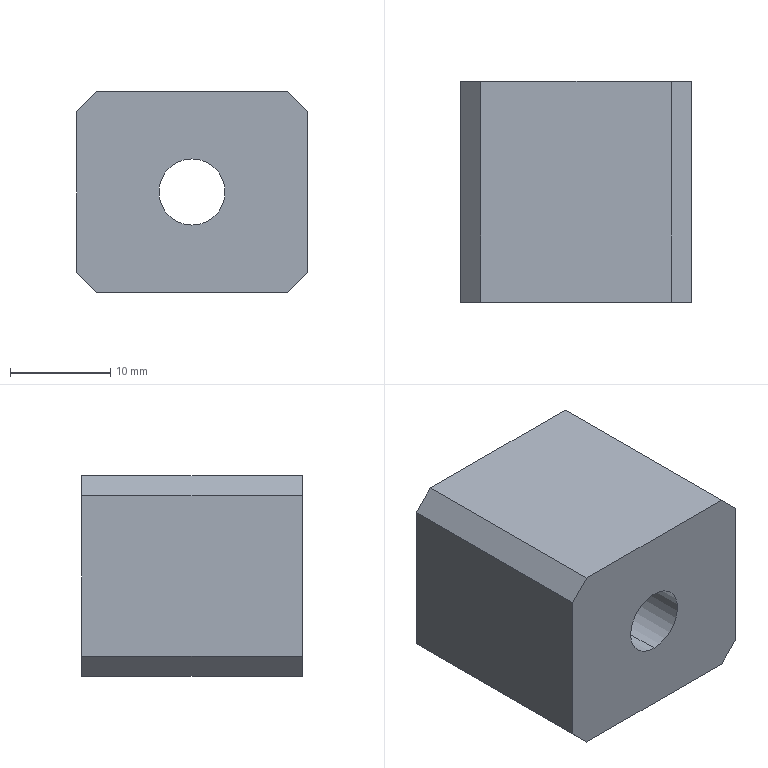Part | SolidWorks | features Chamfer 1, Extrusion 1, HoleWzd 1 | 1 solid | 15 faces | box 23 x 22 x 20 mm | volume 8802 mm3 | plane 11 | cylinder 4 | commonest cylinder face diameters 6.6 x2 11 x2
STEP:
#1=CARTESIAN_POINT('',(0.,4.6,-5.5));
#2=VERTEX_POINT('',#1);
#3=CARTESIAN_POINT('',(0.,4.6,5.5));
#4=VERTEX_POINT('',#3);
#5=CARTESIAN_POINT('',(0.,4.6,0.));
#6=DIRECTION('',(0.,1.,0.));
#7=DIRECTION('',(0.,0.,1.));
#8=AXIS2_PLACEMENT_3D('',#5,#6,#7);
#9=CIRCLE('',#8,5.5);
#10=EDGE_CURVE('',#2,#4,#9,.T.);
#11=ORIENTED_EDGE('',*,*,#10,.F.);
#12=CARTESIAN_POINT('',(0.,11.,-5.5));
#13=VERTEX_POINT('',#12);
#14=CARTESIAN_POINT('',(0.,11.,-5.5));
#15=DIRECTION('',(0.,1.,0.));
#16=VECTOR('',#15,1000.);
#17=LINE('',#14,#16);
#18=EDGE_CURVE('',#2,#13,#17,.T.);
#19=ORIENTED_EDGE('',*,*,#18,.T.);
#20=CARTESIAN_POINT('',(0.,11.,5.5));
#21=VERTEX_POINT('',#20);
#22=CARTESIAN_POINT('',(0.,11.,0.));
#23=DIRECTION('',(0.,1.,0.));
#24=DIRECTION('',(0.,0.,1.));
#25=AXIS2_PLACEMENT_3D('',#22,#23,#24);
#26=CIRCLE('',#25,5.5);
#27=EDGE_CURVE('',#13,#21,#26,.T.);
#28=ORIENTED_EDGE('',*,*,#27,.T.);
#29=CARTESIAN_POINT('',(0.,11.,5.5));
#30=DIRECTION('',(0.,1.,0.));
#31=VECTOR('',#30,1000.);
#32=LINE('',#29,#31);
#33=EDGE_CURVE('',#4,#21,#32,.T.);
#34=ORIENTED_EDGE('',*,*,#33,.F.);
#35=EDGE_LOOP('',(#11,#19,#28,#34));
#36=FACE_OUTER_BOUND('',#35,.T.);
#37=CARTESIAN_POINT('',(0.,11.,0.));
#38=DIRECTION('',(0.,1.,0.));
#39=DIRECTION('',(0.,0.,1.));
#40=AXIS2_PLACEMENT_3D('',#37,#38,#39);
#41=CYLINDRICAL_SURFACE('',#40,5.5);
#42=ADVANCED_FACE('',(#36),#41,.F.);
#43=CARTESIAN_POINT('',(0.,-11.,-3.3));
#44=VERTEX_POINT('',#43);
#45=CARTESIAN_POINT('',(0.,-11.,3.3));
#46=VERTEX_POINT('',#45);
#47=CARTESIAN_POINT('',(0.,-11.,0.));
#48=DIRECTION('',(0.,1.,0.));
#49=DIRECTION('',(0.,0.,1.));
#50=AXIS2_PLACEMENT_3D('',#47,#48,#49);
#51=CIRCLE('',#50,3.3);
#52=EDGE_CURVE('',#44,#46,#51,.T.);
#53=ORIENTED_EDGE('',*,*,#52,.F.);
#54=CARTESIAN_POINT('',(0.,4.6,-3.3));
#55=VERTEX_POINT('',#54);
#56=CARTESIAN_POINT('',(0.,11.,-3.3));
#57=DIRECTION('',(0.,1.,0.));
#58=VECTOR('',#57,1000.);
#59=LINE('',#56,#58);
#60=EDGE_CURVE('',#44,#55,#59,.T.);
#61=ORIENTED_EDGE('',*,*,#60,.T.);
#62=CARTESIAN_POINT('',(0.,4.6,3.3));
#63=VERTEX_POINT('',#62);
#64=CARTESIAN_POINT('',(0.,4.6,0.));
#65=DIRECTION('',(0.,1.,0.));
#66=DIRECTION('',(0.,0.,1.));
#67=AXIS2_PLACEMENT_3D('',#64,#65,#66);
#68=CIRCLE('',#67,3.3);
#69=EDGE_CURVE('',#55,#63,#68,.T.);
#70=ORIENTED_EDGE('',*,*,#69,.T.);
#71=CARTESIAN_POINT('',(0.,11.,3.3));
#72=DIRECTION('',(0.,1.,0.));
#73=VECTOR('',#72,1000.);
#74=LINE('',#71,#73);
#75=EDGE_CURVE('',#46,#63,#74,.T.);
#76=ORIENTED_EDGE('',*,*,#75,.F.);
#77=EDGE_LOOP('',(#53,#61,#70,#76));
#78=FACE_OUTER_BOUND('',#77,.T.);
#79=CARTESIAN_POINT('',(0.,11.,0.));
#80=DIRECTION('',(0.,1.,0.));
#81=DIRECTION('',(0.,0.,1.));
#82=AXIS2_PLACEMENT_3D('',#79,#80,#81);
#83=CYLINDRICAL_SURFACE('',#82,3.3);
#84=ADVANCED_FACE('',(#78),#83,.F.);
#85=CARTESIAN_POINT('',(-11.5,-11.,-8.));
#86=VERTEX_POINT('',#85);
#87=CARTESIAN_POINT('',(-11.5,-11.,8.));
#88=VERTEX_POINT('',#87);
#89=CARTESIAN_POINT('',(-11.5,-11.,-10.));
#90=DIRECTION('',(0.,0.,1.));
#91=VECTOR('',#90,1000.);
#92=LINE('',#89,#91);
#93=EDGE_CURVE('',#86,#88,#92,.T.);
#94=ORIENTED_EDGE('',*,*,#93,.T.);
#95=CARTESIAN_POINT('',(-11.5,11.,8.));
#96=VERTEX_POINT('',#95);
#97=CARTESIAN_POINT('',(-11.5,11.,8.));
#98=DIRECTION('',(0.,1.,0.));
#99=VECTOR('',#98,1000.);
#100=LINE('',#97,#99);
#101=EDGE_CURVE('',#88,#96,#100,.T.);
#102=ORIENTED_EDGE('',*,*,#101,.T.);
#103=CARTESIAN_POINT('',(-11.5,11.,-8.));
#104=VERTEX_POINT('',#103);
#105=CARTESIAN_POINT('',(-11.5,11.,-10.));
#106=DIRECTION('',(0.,0.,1.));
#107=VECTOR('',#106,1000.);
#108=LINE('',#105,#107);
#109=EDGE_CURVE('',#104,#96,#108,.T.);
#110=ORIENTED_EDGE('',*,*,#109,.F.);
#111=CARTESIAN_POINT('',(-11.5,11.,-8.));
#112=DIRECTION('',(0.,-1.,0.));
#113=VECTOR('',#112,1000.);
#114=LINE('',#111,#113);
#115=EDGE_CURVE('',#104,#86,#114,.T.);
#116=ORIENTED_EDGE('',*,*,#115,.T.);
#117=EDGE_LOOP('',(#94,#102,#110,#116));
#118=FACE_OUTER_BOUND('',#117,.T.);
#119=CARTESIAN_POINT('',(-11.5,11.,-10.));
#120=DIRECTION('',(1.,0.,0.));
#121=DIRECTION('',(0.,0.,-1.));
#122=AXIS2_PLACEMENT_3D('',#119,#120,#121);
#123=PLANE('',#122);
#124=ADVANCED_FACE('',(#118),#123,.F.);
#125=CARTESIAN_POINT('',(-9.5,-11.,10.));
#126=VERTEX_POINT('',#125);
#127=CARTESIAN_POINT('',(9.5,-11.,10.));
#128=VERTEX_POINT('',#127);
#129=CARTESIAN_POINT('',(-11.5,-11.,10.));
#130=DIRECTION('',(1.,0.,0.));
#131=VECTOR('',#130,1000.);
#132=LINE('',#129,#131);
#133=EDGE_CURVE('',#126,#128,#132,.T.);
#134=ORIENTED_EDGE('',*,*,#133,.T.);
#135=CARTESIAN_POINT('',(9.5,11.,10.));
#136=VERTEX_POINT('',#135);
#137=CARTESIAN_POINT('',(9.5,11.,10.));
#138=DIRECTION('',(0.,1.,0.));
#139=VECTOR('',#138,1000.);
#140=LINE('',#137,#139);
#141=EDGE_CURVE('',#128,#136,#140,.T.);
#142=ORIENTED_EDGE('',*,*,#141,.T.);
#143=CARTESIAN_POINT('',(-9.5,11.,10.));
#144=VERTEX_POINT('',#143);
#145=CARTESIAN_POINT('',(-11.5,11.,10.));
#146=DIRECTION('',(1.,0.,0.));
#147=VECTOR('',#146,1000.);
#148=LINE('',#145,#147);
#149=EDGE_CURVE('',#144,#136,#148,.T.);
#150=ORIENTED_EDGE('',*,*,#149,.F.);
#151=CARTESIAN_POINT('',(-9.5,11.,10.));
#152=DIRECTION('',(0.,-1.,0.));
#153=VECTOR('',#152,1000.);
#154=LINE('',#151,#153);
#155=EDGE_CURVE('',#144,#126,#154,.T.);
#156=ORIENTED_EDGE('',*,*,#155,.T.);
#157=EDGE_LOOP('',(#134,#142,#150,#156));
#158=FACE_OUTER_BOUND('',#157,.T.);
#159=CARTESIAN_POINT('',(-11.5,11.,10.));
#160=DIRECTION('',(0.,0.,-1.));
#161=DIRECTION('',(-1.,0.,0.));
#162=AXIS2_PLACEMENT_3D('',#159,#160,#161);
#163=PLANE('',#162);
#164=ADVANCED_FACE('',(#158),#163,.F.);
#165=CARTESIAN_POINT('',(11.5,11.,8.));
#166=VERTEX_POINT('',#165);
#167=CARTESIAN_POINT('',(11.5,11.,-8.));
#168=VERTEX_POINT('',#167);
#169=CARTESIAN_POINT('',(11.5,11.,-10.));
#170=DIRECTION('',(0.,0.,-1.));
#171=VECTOR('',#170,1000.);
#172=LINE('',#169,#171);
#173=EDGE_CURVE('',#166,#168,#172,.T.);
#174=ORIENTED_EDGE('',*,*,#173,.F.);
#175=CARTESIAN_POINT('',(11.5,-11.,8.));
#176=VERTEX_POINT('',#175);
#177=CARTESIAN_POINT('',(11.5,11.,8.));
#178=DIRECTION('',(0.,-1.,0.));
#179=VECTOR('',#178,1000.);
#180=LINE('',#177,#179);
#181=EDGE_CURVE('',#166,#176,#180,.T.);
#182=ORIENTED_EDGE('',*,*,#181,.T.);
#183=CARTESIAN_POINT('',(11.5,-11.,-8.));
#184=VERTEX_POINT('',#183);
#185=CARTESIAN_POINT('',(11.5,-11.,-10.));
#186=DIRECTION('',(0.,0.,-1.));
#187=VECTOR('',#186,1000.);
#188=LINE('',#185,#187);
#189=EDGE_CURVE('',#176,#184,#188,.T.);
#190=ORIENTED_EDGE('',*,*,#189,.T.);
#191=CARTESIAN_POINT('',(11.5,11.,-8.));
#192=DIRECTION('',(0.,1.,0.));
#193=VECTOR('',#192,1000.);
#194=LINE('',#191,#193);
#195=EDGE_CURVE('',#184,#168,#194,.T.);
#196=ORIENTED_EDGE('',*,*,#195,.T.);
#197=EDGE_LOOP('',(#174,#182,#190,#196));
#198=FACE_OUTER_BOUND('',#197,.T.);
#199=CARTESIAN_POINT('',(11.5,11.,-10.));
#200=DIRECTION('',(-1.,0.,0.));
#201=DIRECTION('',(0.,0.,1.));
#202=AXIS2_PLACEMENT_3D('',#199,#200,#201);
#203=PLANE('',#202);
#204=ADVANCED_FACE('',(#198),#203,.F.);
#205=CARTESIAN_POINT('',(9.5,11.,-10.));
#206=VERTEX_POINT('',#205);
#207=CARTESIAN_POINT('',(-9.5,11.,-10.));
#208=VERTEX_POINT('',#207);
#209=CARTESIAN_POINT('',(-11.5,11.,-10.));
#210=DIRECTION('',(-1.,0.,0.));
#211=VECTOR('',#210,1000.);
#212=LINE('',#209,#211);
#213=EDGE_CURVE('',#206,#208,#212,.T.);
#214=ORIENTED_EDGE('',*,*,#213,.F.);
#215=CARTESIAN_POINT('',(9.5,-11.,-10.));
#216=VERTEX_POINT('',#215);
#217=CARTESIAN_POINT('',(9.5,11.,-10.));
#218=DIRECTION('',(0.,-1.,0.));
#219=VECTOR('',#218,1000.);
#220=LINE('',#217,#219);
#221=EDGE_CURVE('',#206,#216,#220,.T.);
#222=ORIENTED_EDGE('',*,*,#221,.T.);
#223=CARTESIAN_POINT('',(-9.5,-11.,-10.));
#224=VERTEX_POINT('',#223);
#225=CARTESIAN_POINT('',(-11.5,-11.,-10.));
#226=DIRECTION('',(-1.,0.,0.));
#227=VECTOR('',#226,1000.);
#228=LINE('',#225,#227);
#229=EDGE_CURVE('',#216,#224,#228,.T.);
#230=ORIENTED_EDGE('',*,*,#229,.T.);
#231=CARTESIAN_POINT('',(-9.5,11.,-10.));
#232=DIRECTION('',(0.,1.,0.));
#233=VECTOR('',#232,1000.);
#234=LINE('',#231,#233);
#235=EDGE_CURVE('',#224,#208,#234,.T.);
#236=ORIENTED_EDGE('',*,*,#235,.T.);
#237=EDGE_LOOP('',(#214,#222,#230,#236));
#238=FACE_OUTER_BOUND('',#237,.T.);
#239=CARTESIAN_POINT('',(-11.5,11.,-10.));
#240=DIRECTION('',(0.,0.,1.));
#241=DIRECTION('',(1.,0.,0.));
#242=AXIS2_PLACEMENT_3D('',#239,#240,#241);
#243=PLANE('',#242);
#244=ADVANCED_FACE('',(#238),#243,.F.);
#245=CARTESIAN_POINT('',(0.,11.,0.));
#246=DIRECTION('',(0.,1.,0.));
#247=DIRECTION('',(0.,0.,1.));
#248=AXIS2_PLACEMENT_3D('',#245,#246,#247);
#249=CIRCLE('',#248,5.5);
#250=EDGE_CURVE('',#21,#13,#249,.T.);
#251=ORIENTED_EDGE('',*,*,#250,.F.);
#252=ORIENTED_EDGE('',*,*,#27,.F.);
#253=EDGE_LOOP('',(#251,#252));
#254=FACE_BOUND('',#253,.T.);
#255=ORIENTED_EDGE('',*,*,#149,.T.);
#256=CARTESIAN_POINT('',(9.75,11.,9.75));
#257=DIRECTION('',(0.7071,0.,-0.7071));
#258=VECTOR('',#257,1000.);
#259=LINE('',#256,#258);
#260=EDGE_CURVE('',#136,#166,#259,.T.);
#261=ORIENTED_EDGE('',*,*,#260,.T.);
#262=ORIENTED_EDGE('',*,*,#173,.T.);
#263=CARTESIAN_POINT('',(9.75,11.,-9.75));
#264=DIRECTION('',(-0.7071,0.,-0.7071));
#265=VECTOR('',#264,1000.);
#266=LINE('',#263,#265);
#267=EDGE_CURVE('',#168,#206,#266,.T.);
#268=ORIENTED_EDGE('',*,*,#267,.T.);
#269=ORIENTED_EDGE('',*,*,#213,.T.);
#270=CARTESIAN_POINT('',(-9.75,11.,-9.75));
#271=DIRECTION('',(-0.7071,0.,0.7071));
#272=VECTOR('',#271,1000.);
#273=LINE('',#270,#272);
#274=EDGE_CURVE('',#208,#104,#273,.T.);
#275=ORIENTED_EDGE('',*,*,#274,.T.);
#276=ORIENTED_EDGE('',*,*,#109,.T.);
#277=CARTESIAN_POINT('',(-9.75,11.,9.75));
#278=DIRECTION('',(0.7071,0.,0.7071));
#279=VECTOR('',#278,1000.);
#280=LINE('',#277,#279);
#281=EDGE_CURVE('',#96,#144,#280,.T.);
#282=ORIENTED_EDGE('',*,*,#281,.T.);
#283=EDGE_LOOP('',(#255,#261,#262,#268,#269,#275,#276,#282));
#284=FACE_OUTER_BOUND('',#283,.T.);
#285=CARTESIAN_POINT('',(0.,11.,0.));
#286=DIRECTION('',(0.,1.,0.));
#287=DIRECTION('',(0.,0.,1.));
#288=AXIS2_PLACEMENT_3D('',#285,#286,#287);
#289=PLANE('',#288);
#290=ADVANCED_FACE('',(#254,#284),#289,.T.);
#291=CARTESIAN_POINT('',(0.,-11.,0.));
#292=DIRECTION('',(0.,1.,0.));
#293=DIRECTION('',(0.,0.,1.));
#294=AXIS2_PLACEMENT_3D('',#291,#292,#293);
#295=CIRCLE('',#294,3.3);
#296=EDGE_CURVE('',#46,#44,#295,.T.);
#297=ORIENTED_EDGE('',*,*,#296,.T.);
#298=ORIENTED_EDGE('',*,*,#52,.T.);
#299=EDGE_LOOP('',(#297,#298));
#300=FACE_BOUND('',#299,.T.);
#301=ORIENTED_EDGE('',*,*,#189,.F.);
#302=CARTESIAN_POINT('',(11.5,-11.,8.));
#303=DIRECTION('',(-0.7071,0.,0.7071));
#304=VECTOR('',#303,1000.);
#305=LINE('',#302,#304);
#306=EDGE_CURVE('',#176,#128,#305,.T.);
#307=ORIENTED_EDGE('',*,*,#306,.T.);
#308=ORIENTED_EDGE('',*,*,#133,.F.);
#309=CARTESIAN_POINT('',(-9.5,-11.,10.));
#310=DIRECTION('',(-0.7071,0.,-0.7071));
#311=VECTOR('',#310,1000.);
#312=LINE('',#309,#311);
#313=EDGE_CURVE('',#126,#88,#312,.T.);
#314=ORIENTED_EDGE('',*,*,#313,.T.);
#315=ORIENTED_EDGE('',*,*,#93,.F.);
#316=CARTESIAN_POINT('',(-11.5,-11.,-8.));
#317=DIRECTION('',(0.7071,0.,-0.7071));
#318=VECTOR('',#317,1000.);
#319=LINE('',#316,#318);
#320=EDGE_CURVE('',#86,#224,#319,.T.);
#321=ORIENTED_EDGE('',*,*,#320,.T.);
#322=ORIENTED_EDGE('',*,*,#229,.F.);
#323=CARTESIAN_POINT('',(9.5,-11.,-10.));
#324=DIRECTION('',(0.7071,0.,0.7071));
#325=VECTOR('',#324,1000.);
#326=LINE('',#323,#325);
#327=EDGE_CURVE('',#216,#184,#326,.T.);
#328=ORIENTED_EDGE('',*,*,#327,.T.);
#329=EDGE_LOOP('',(#301,#307,#308,#314,#315,#321,#322,#328));
#330=FACE_OUTER_BOUND('',#329,.T.);
#331=CARTESIAN_POINT('',(0.,-11.,0.));
#332=DIRECTION('',(0.,1.,0.));
#333=DIRECTION('',(0.,0.,1.));
#334=AXIS2_PLACEMENT_3D('',#331,#332,#333);
#335=PLANE('',#334);
#336=ADVANCED_FACE('',(#300,#330),#335,.F.);
#337=ORIENTED_EDGE('',*,*,#60,.F.);
#338=ORIENTED_EDGE('',*,*,#296,.F.);
#339=ORIENTED_EDGE('',*,*,#75,.T.);
#340=CARTESIAN_POINT('',(0.,4.6,0.));
#341=DIRECTION('',(0.,1.,0.));
#342=DIRECTION('',(0.,0.,1.));
#343=AXIS2_PLACEMENT_3D('',#340,#341,#342);
#344=CIRCLE('',#343,3.3);
#345=EDGE_CURVE('',#63,#55,#344,.T.);
#346=ORIENTED_EDGE('',*,*,#345,.T.);
#347=EDGE_LOOP('',(#337,#338,#339,#346));
#348=FACE_OUTER_BOUND('',#347,.T.);
#349=CARTESIAN_POINT('',(0.,11.,0.));
#350=DIRECTION('',(0.,1.,0.));
#351=DIRECTION('',(0.,0.,1.));
#352=AXIS2_PLACEMENT_3D('',#349,#350,#351);
#353=CYLINDRICAL_SURFACE('',#352,3.3);
#354=ADVANCED_FACE('',(#348),#353,.F.);
#355=ORIENTED_EDGE('',*,*,#345,.F.);
#356=ORIENTED_EDGE('',*,*,#69,.F.);
#357=EDGE_LOOP('',(#355,#356));
#358=FACE_BOUND('',#357,.T.);
#359=CARTESIAN_POINT('',(0.,4.6,0.));
#360=DIRECTION('',(0.,1.,0.));
#361=DIRECTION('',(0.,0.,1.));
#362=AXIS2_PLACEMENT_3D('',#359,#360,#361);
#363=CIRCLE('',#362,5.5);
#364=EDGE_CURVE('',#4,#2,#363,.T.);
#365=ORIENTED_EDGE('',*,*,#364,.T.);
#366=ORIENTED_EDGE('',*,*,#10,.T.);
#367=EDGE_LOOP('',(#365,#366));
#368=FACE_OUTER_BOUND('',#367,.T.);
#369=CARTESIAN_POINT('',(3.3,4.6,0.));
#370=DIRECTION('',(0.,-1.,0.));
#371=DIRECTION('',(0.,0.,-1.));
#372=AXIS2_PLACEMENT_3D('',#369,#370,#371);
#373=PLANE('',#372);
#374=ADVANCED_FACE('',(#358,#368),#373,.F.);
#375=ORIENTED_EDGE('',*,*,#18,.F.);
#376=ORIENTED_EDGE('',*,*,#364,.F.);
#377=ORIENTED_EDGE('',*,*,#33,.T.);
#378=ORIENTED_EDGE('',*,*,#250,.T.);
#379=EDGE_LOOP('',(#375,#376,#377,#378));
#380=FACE_OUTER_BOUND('',#379,.T.);
#381=CARTESIAN_POINT('',(0.,11.,0.));
#382=DIRECTION('',(0.,1.,0.));
#383=DIRECTION('',(0.,0.,1.));
#384=AXIS2_PLACEMENT_3D('',#381,#382,#383);
#385=CYLINDRICAL_SURFACE('',#384,5.5);
#386=ADVANCED_FACE('',(#380),#385,.F.);
#387=ORIENTED_EDGE('',*,*,#260,.F.);
#388=ORIENTED_EDGE('',*,*,#141,.F.);
#389=ORIENTED_EDGE('',*,*,#306,.F.);
#390=ORIENTED_EDGE('',*,*,#181,.F.);
#391=EDGE_LOOP('',(#387,#388,#389,#390));
#392=FACE_OUTER_BOUND('',#391,.T.);
#393=CARTESIAN_POINT('',(11.5,11.,8.));
#394=DIRECTION('',(-0.7071,0.,-0.7071));
#395=DIRECTION('',(0.,-1.,0.));
#396=AXIS2_PLACEMENT_3D('',#393,#394,#395);
#397=PLANE('',#396);
#398=ADVANCED_FACE('',(#392),#397,.F.);
#399=ORIENTED_EDGE('',*,*,#281,.F.);
#400=ORIENTED_EDGE('',*,*,#101,.F.);
#401=ORIENTED_EDGE('',*,*,#313,.F.);
#402=ORIENTED_EDGE('',*,*,#155,.F.);
#403=EDGE_LOOP('',(#399,#400,#401,#402));
#404=FACE_OUTER_BOUND('',#403,.T.);
#405=CARTESIAN_POINT('',(-9.5,11.,10.));
#406=DIRECTION('',(0.7071,0.,-0.7071));
#407=DIRECTION('',(0.,-1.,0.));
#408=AXIS2_PLACEMENT_3D('',#405,#406,#407);
#409=PLANE('',#408);
#410=ADVANCED_FACE('',(#404),#409,.F.);
#411=ORIENTED_EDGE('',*,*,#267,.F.);
#412=ORIENTED_EDGE('',*,*,#195,.F.);
#413=ORIENTED_EDGE('',*,*,#327,.F.);
#414=ORIENTED_EDGE('',*,*,#221,.F.);
#415=EDGE_LOOP('',(#411,#412,#413,#414));
#416=FACE_OUTER_BOUND('',#415,.T.);
#417=CARTESIAN_POINT('',(9.5,11.,-10.));
#418=DIRECTION('',(-0.7071,0.,0.7071));
#419=DIRECTION('',(0.,-1.,0.));
#420=AXIS2_PLACEMENT_3D('',#417,#418,#419);
#421=PLANE('',#420);
#422=ADVANCED_FACE('',(#416),#421,.F.);
#423=ORIENTED_EDGE('',*,*,#274,.F.);
#424=ORIENTED_EDGE('',*,*,#235,.F.);
#425=ORIENTED_EDGE('',*,*,#320,.F.);
#426=ORIENTED_EDGE('',*,*,#115,.F.);
#427=EDGE_LOOP('',(#423,#424,#425,#426));
#428=FACE_OUTER_BOUND('',#427,.T.);
#429=CARTESIAN_POINT('',(-11.5,11.,-8.));
#430=DIRECTION('',(0.7071,0.,0.7071));
#431=DIRECTION('',(0.,-1.,0.));
#432=AXIS2_PLACEMENT_3D('',#429,#430,#431);
#433=PLANE('',#432);
#434=ADVANCED_FACE('',(#428),#433,.F.);
#435=CLOSED_SHELL('',(#42,#84,#124,#164,#204,#244,#290,#336,#354,#374,#386,#398,#410,#422,#434));
#436=MANIFOLD_SOLID_BREP('',#435);
#437=CARTESIAN_POINT('',(0.,0.,0.));
#438=DIRECTION('',(0.,0.,1.));
#439=DIRECTION('',(1.,0.,0.));
#440=AXIS2_PLACEMENT_3D('',#437,#438,#439);
#441=(LENGTH_UNIT()NAMED_UNIT(*)SI_UNIT(.MILLI.,.METRE.));
#442=UNCERTAINTY_MEASURE_WITH_UNIT(LENGTH_MEASURE(0.00001),#441,'','');
#443=(NAMED_UNIT(*)PLANE_ANGLE_UNIT()SI_UNIT($,.RADIAN.));
#444=(NAMED_UNIT(*)SI_UNIT($,.STERADIAN.)SOLID_ANGLE_UNIT());
#445=(GEOMETRIC_REPRESENTATION_CONTEXT(3)GLOBAL_UNCERTAINTY_ASSIGNED_CONTEXT((#442))GLOBAL_UNIT_ASSIGNED_CONTEXT((#441,#443,#444))REPRESENTATION_CONTEXT('',''));
#446=ADVANCED_BREP_SHAPE_REPRESENTATION('',(#436,#440),#445);